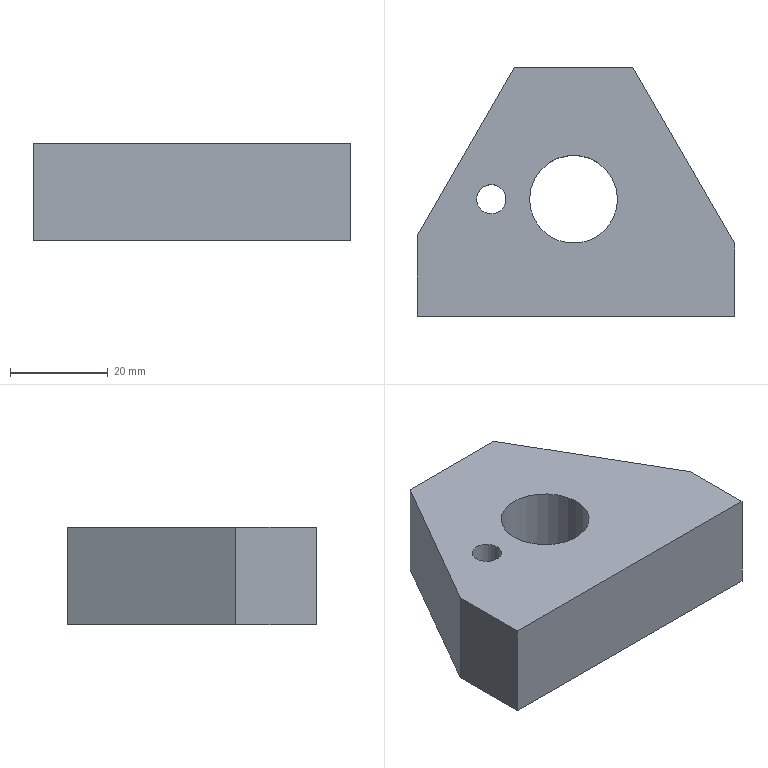CAM job | NX | 3+2 milling, drilling | part box 65 x 51 x 20 mm | stock box 65 x 54 x 20 mm
Tools:
number,name,description,diameter,corner_radius,flute_length,length,flutes
2,D8,Milling Tool-5 Parameters,8.0,0.0,50.0,75.0,2
12,D4平刀,Milling Tool-5 Parameters,4.0,0.0,50.0,75.0,2
Operations:
program,operation,operation_type,tool,method,geometry_group,spindle_rpm,surface_speed,feed_per_tooth,feed_cut,feed_plunge,cut_length_mm,path_length_mm,cut_time_min,machine_time_min
G54,ADAPTIVE_MILLING,CavityMilling,D8,METHOD,WORKPIECE,5500.0,138.0,0.2273,2500.0,100.0,2785.602,3109.612,1.112,1.145
G54,PLANAR_MILL_COPY,PlanarMilling,D8,METHOD,WORKPIECE,4500.0,113.0,0.0667,600.0,100.0,40.043,94.043,0.0667,0.0721
G54,PLANAR_MILL,PlanarMilling,D8,METHOD,WORKPIECE,4500.0,113.0,0.0667,600.0,100.0,240.563,294.563,0.4009,0.4063
G54,DRILLING,Operation,D8,METHOD,WORKPIECE,0.0,0.0,0.0,250.0,0.0,3.0,9.0,0.012,0.0126
G55,PLANAR_MILL_1,PlanarMilling,D4平刀,METHOD,MCS,3500.0,43.0,0.0714,500.0,100.0,494.764,494.764,0.9895,0.9895
G55,PLANAR_MILL_1_COPY,PlanarMilling,D4平刀,METHOD,MCS,3000.0,37.0,0.05,300.0,100.0,14.297,14.297,0.0477,0.0477